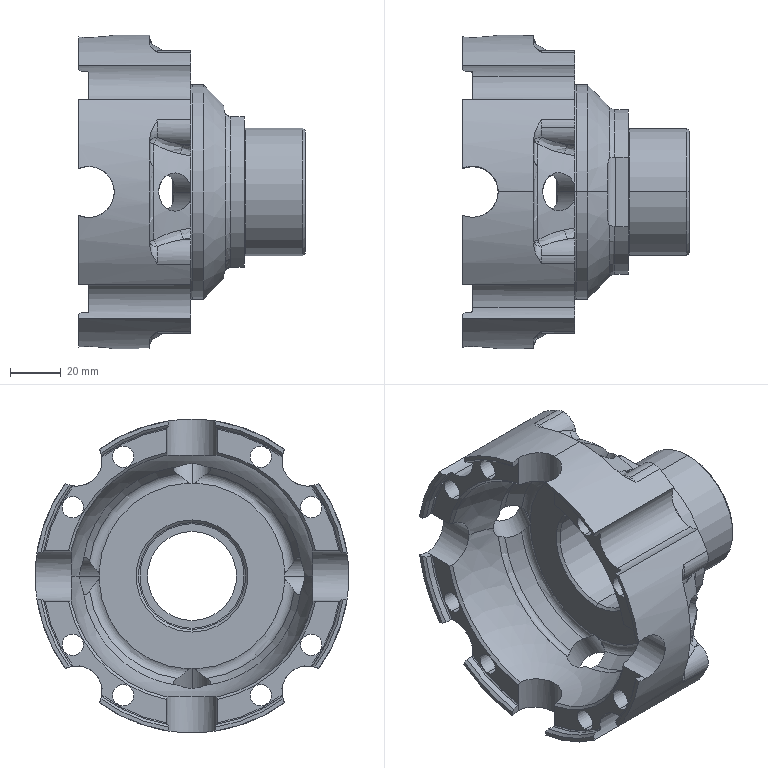Part | SolidWorks | features Cut 5, Fillet 3, CirPattern 2, Chamfer 1, RevCut 1, Revolution 1 | 1 solid | 212 faces | box 89 x 123 x 123 mm | volume 266292 mm3 | cylinder 79 | torus 41 | plane 34 | cone 28 | spline 16 | sphere 14 | commonest cylinder face diameters 20 x18 8.4 x16 14 x10 15 x8 118 x8 123 x5